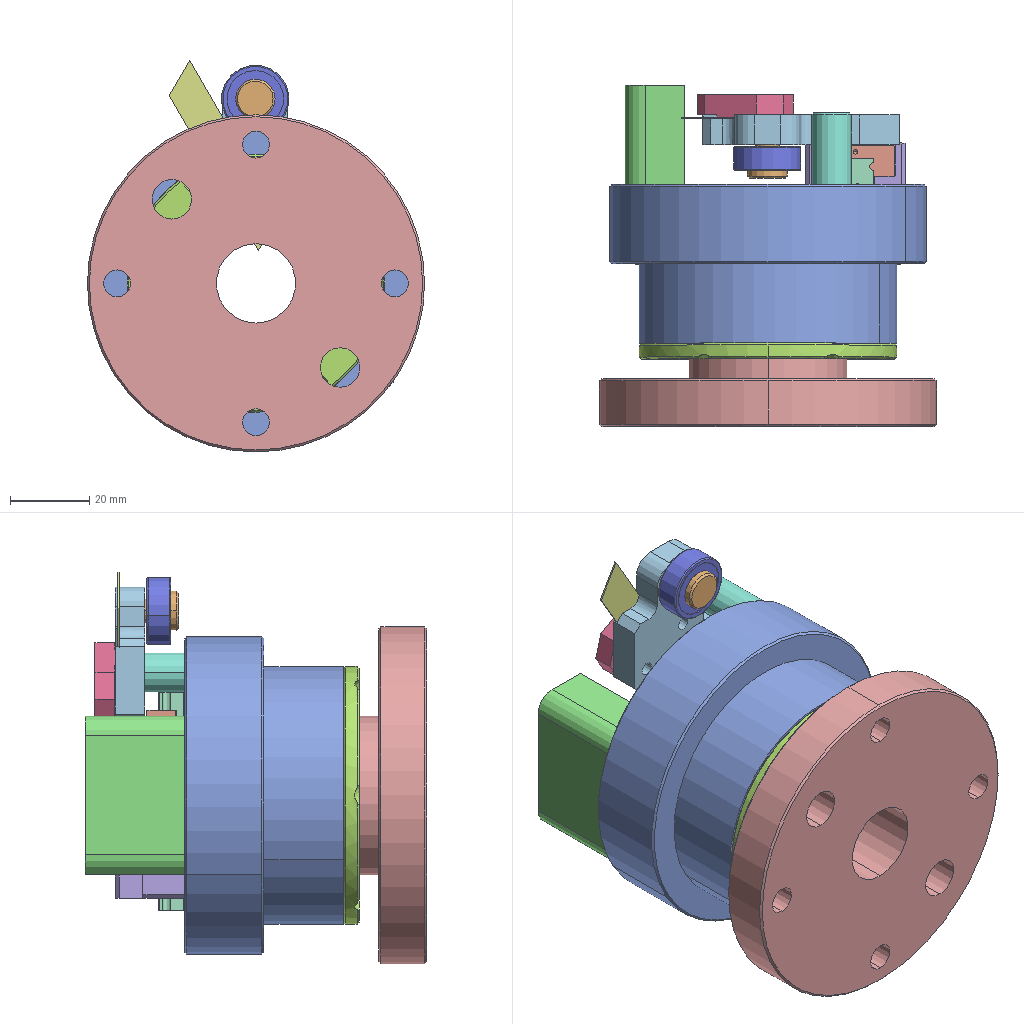Assembly | SolidWorks | 14 different items | 14 placed | box 85 x 86 x 99 mm
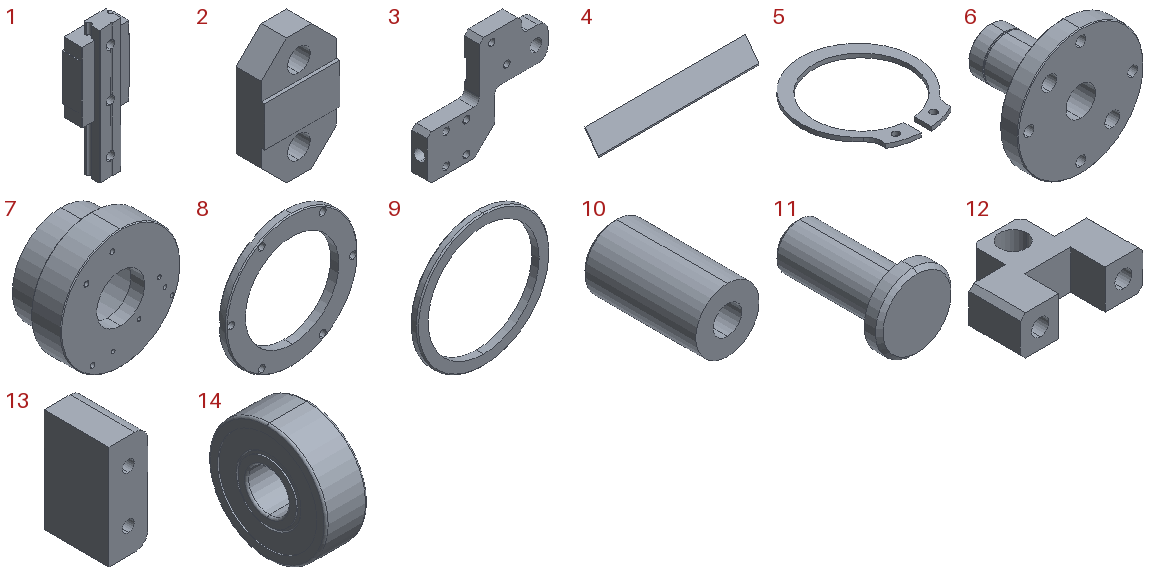Parts list (item | name | quantity | size | volume | features):
1 | (subassembly) | x1 | 20 x 10 x 55 mm | 5950 mm3 | -
2 | - | x1 | 15 x 5.7 x 25 mm | 1550 mm3 | features Chamfer 1, Extrusion 1, HoleWzd 1, ICE 1
3 | - | x1 | 60 x 7.5 x 49.5 mm | 9409 mm3 | features HoleWzd 3, ICE 3, Chamfer 2, Fillet 2, Extrusion 1
4 | - | x1 | 50.196 x 9 x 0.4 mm | 162 mm3 | features Extrusion 1
5 | - | x1 | 33.5 x 36.623 x 1.2 mm | 375.357 mm3 | features MBimport 1
6 | - | x1 | 85 x 61 x 85 mm | 84723 mm3 | features HoleWzd 2, Chamfer 1, ICE 1, RevCut 1, Revolution 1
7 | - | x1 | 80 x 40 x 80 mm | 86830 mm3 | features HoleWzd 5, Chamfer 1, RevCut 1, Revolution 1
8 | - | x1 | 65 x 4 x 65 mm | 6250 mm3 | features Chamfer 1, Extrusion 1, HoleWzd 1
9 | - | x1 | 55 x 3 x 55 mm | 2099 mm3 | features Chamfer 1, Extrusion 1
10 | - | x1 | 10 x 18 x 10 mm | 965.582 mm3 | features Chamfer 1, Extrusion 1, HoleWzd 1
11 | - | x1 | 10 x 16 x 10 mm | 546.899 mm3 | features Chamfer 1, Extrusion 1, ICE 1
12 | - | x1 | 25 x 17.5 x 8 mm | 1778 mm3 | features ICE 3, Chamfer 1, Extrusion 1, HoleWzd 1
13 | - | x1 | 15 x 25 x 40 mm | 13620 mm3 | features Extrusion 1, Fillet 1, HoleWzd 1
14 | - | x1 | 6 x 17 x 17 mm | 1023 mm3 | features BaseBody 1
Mates (type | each side: item.copy, entity, surface, feature):
Concentric | 7.1 face cylinder Revolve1 | 8.1 face cylinder Boss-Extrude1
Concentric | 7.1 face cylinder M3 Tapped Hole1 | 8.1 face cylinder Hole wizard: slotted raised countersunk wood screw, type 1
Coincident | 7.1 face plane Revolve1 | 8.1 face plane Boss-Extrude1
Concentric | 6.1 face cylinder Revolve1 | 8.1 face cylinder Boss-Extrude1
DistanceDim | 8.1 face plane Boss-Extrude1 | 6.1 face plane Revolve1
Concentric | 6.1 face cylinder Cut-Revolve1 | 5.1 face cylinder
Coincident | 6.1 face plane Cut-Revolve1 | 5.1 face plane
Parallel | 8.1 plane | assembly plane
Parallel | 5.1 plane | assembly plane
Concentric | 11.1 face cylinder Boss-Extrude2 | 14.1 face cylinder BAG606-2RS-E
Coincident | 11.1 face plane Boss-Extrude1 | 14.1 face plane BAG606-2RS-E
Coincident | 4.1 face plane Boss-Extrude1 | 3.1 face plane Cut-Extrude2
Width | 4.1 face plane Boss-Extrude1 | 4.1 face plane Boss-Extrude1 | 3.1 face plane Cut-Extrude2 | 3.1 face plane Cut-Extrude2
Coincident | 4.1 face plane Boss-Extrude1 | 2.1 face plane Boss-Extrude1
Concentric | 2.1 face cylinder Ø4.5 (4.5) Diameter Hole1 | 3.1 face cylinder M4 Tapped Hole1 | 2 times
Coincident | 7.1 face plane Revolve1 | 13.1 face plane Boss-Extrude1
Coincident | 7.1 face plane Revolve1 | 10.1 face plane Boss-Extrude1
Concentric | 3.1 face cylinder Ø6.0 (6) Diameter Hole1 | 11.1 face cylinder Boss-Extrude2
Coincident | 3.1 face plane Boss-Extrude1 | 11.1 face plane Boss-Extrude2
Coincident | 6.1 plane | 13.1 plane
DistanceDim | 13.1 face plane Boss-Extrude1 | 6.1 plane
Tangent | 10.1 face cylinder Boss-Extrude1 | 3.1 face plane Cut-Extrude1
Parallel | 11.1 plane | 3.1 face plane Cut-Extrude1
Parallel | 10.1 plane | 3.1 face plane Cut-Extrude1
DistanceDim | 10.1 plane | 3.1 face plane Cut-Extrude1